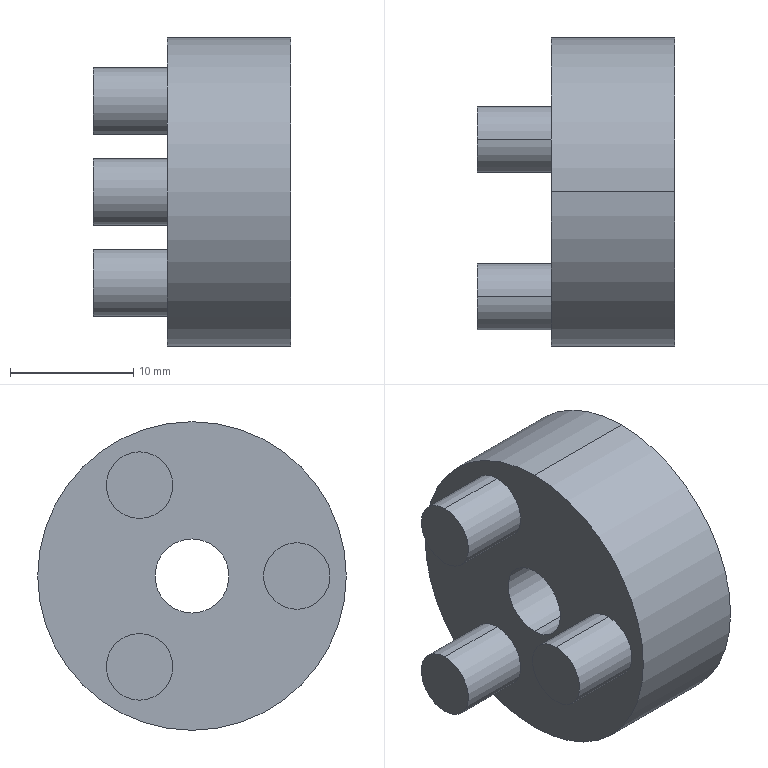Part | SolidWorks | features BaseBody 1 | 1 solid | 15 faces | box 16 x 25 x 25 mm | volume 5038 mm3 | cylinder 10 | plane 5 | commonest cylinder face diameters 5.4 x6 6 x2 25 x2
STEP:
#1=CARTESIAN_POINT('',(5.,0.,12.5));
#2=VERTEX_POINT('',#1);
#3=CARTESIAN_POINT('',(5.,0.,-12.5));
#4=VERTEX_POINT('',#3);
#5=CARTESIAN_POINT('',(5.,0.,0.));
#6=DIRECTION('',(-1.,0.,0.));
#7=DIRECTION('',(0.,0.,1.));
#8=AXIS2_PLACEMENT_3D('',#5,#6,#7);
#9=CIRCLE('',#8,12.5);
#10=EDGE_CURVE('',#2,#4,#9,.T.);
#11=ORIENTED_EDGE('',*,*,#10,.T.);
#12=CARTESIAN_POINT('',(-5.,0.,-12.5));
#13=VERTEX_POINT('',#12);
#14=CARTESIAN_POINT('',(5.,0.,-12.5));
#15=DIRECTION('',(-1.,0.,0.));
#16=VECTOR('',#15,1000.);
#17=LINE('',#14,#16);
#18=EDGE_CURVE('',#4,#13,#17,.T.);
#19=ORIENTED_EDGE('',*,*,#18,.T.);
#20=CARTESIAN_POINT('',(-5.,0.,12.5));
#21=VERTEX_POINT('',#20);
#22=CARTESIAN_POINT('',(-5.,0.,0.));
#23=DIRECTION('',(1.,0.,0.));
#24=DIRECTION('',(0.,0.,1.));
#25=AXIS2_PLACEMENT_3D('',#22,#23,#24);
#26=CIRCLE('',#25,12.5);
#27=EDGE_CURVE('',#13,#21,#26,.T.);
#28=ORIENTED_EDGE('',*,*,#27,.T.);
#29=CARTESIAN_POINT('',(5.,0.,12.5));
#30=DIRECTION('',(-1.,0.,0.));
#31=VECTOR('',#30,1000.);
#32=LINE('',#29,#31);
#33=EDGE_CURVE('',#2,#21,#32,.T.);
#34=ORIENTED_EDGE('',*,*,#33,.F.);
#35=EDGE_LOOP('',(#11,#19,#28,#34));
#36=FACE_OUTER_BOUND('',#35,.T.);
#37=CARTESIAN_POINT('',(5.,0.,0.));
#38=DIRECTION('',(-1.,0.,0.));
#39=DIRECTION('',(0.,0.,1.));
#40=AXIS2_PLACEMENT_3D('',#37,#38,#39);
#41=CYLINDRICAL_SURFACE('',#40,12.5);
#42=ADVANCED_FACE('',(#36),#41,.T.);
#43=CARTESIAN_POINT('',(-5.,0.,3.));
#44=VERTEX_POINT('',#43);
#45=CARTESIAN_POINT('',(-5.,0.,-3.));
#46=VERTEX_POINT('',#45);
#47=CARTESIAN_POINT('',(-5.,0.,0.));
#48=DIRECTION('',(1.,0.,0.));
#49=DIRECTION('',(0.,0.,-1.));
#50=AXIS2_PLACEMENT_3D('',#47,#48,#49);
#51=CIRCLE('',#50,3.);
#52=EDGE_CURVE('',#44,#46,#51,.T.);
#53=ORIENTED_EDGE('',*,*,#52,.F.);
#54=CARTESIAN_POINT('',(5.,0.,3.));
#55=VERTEX_POINT('',#54);
#56=CARTESIAN_POINT('',(-6.,0.,3.));
#57=DIRECTION('',(1.,0.,0.));
#58=VECTOR('',#57,1000.);
#59=LINE('',#56,#58);
#60=EDGE_CURVE('',#44,#55,#59,.T.);
#61=ORIENTED_EDGE('',*,*,#60,.T.);
#62=CARTESIAN_POINT('',(5.,0.,-3.));
#63=VERTEX_POINT('',#62);
#64=CARTESIAN_POINT('',(5.,0.,0.));
#65=DIRECTION('',(1.,0.,0.));
#66=DIRECTION('',(0.,0.,-1.));
#67=AXIS2_PLACEMENT_3D('',#64,#65,#66);
#68=CIRCLE('',#67,3.);
#69=EDGE_CURVE('',#55,#63,#68,.T.);
#70=ORIENTED_EDGE('',*,*,#69,.T.);
#71=CARTESIAN_POINT('',(-6.,0.,-3.));
#72=DIRECTION('',(1.,0.,0.));
#73=VECTOR('',#72,1000.);
#74=LINE('',#71,#73);
#75=EDGE_CURVE('',#46,#63,#74,.T.);
#76=ORIENTED_EDGE('',*,*,#75,.F.);
#77=EDGE_LOOP('',(#53,#61,#70,#76));
#78=FACE_OUTER_BOUND('',#77,.T.);
#79=CARTESIAN_POINT('',(-6.,0.,0.));
#80=DIRECTION('',(1.,0.,0.));
#81=DIRECTION('',(0.,0.,-1.));
#82=AXIS2_PLACEMENT_3D('',#79,#80,#81);
#83=CYLINDRICAL_SURFACE('',#82,3.);
#84=ADVANCED_FACE('',(#78),#83,.F.);
#85=CARTESIAN_POINT('',(-5.,4.25,-10.061));
#86=VERTEX_POINT('',#85);
#87=CARTESIAN_POINT('',(-5.,4.25,-4.661));
#88=VERTEX_POINT('',#87);
#89=CARTESIAN_POINT('',(-5.,4.25,-7.361));
#90=DIRECTION('',(1.,0.,0.));
#91=DIRECTION('',(0.,0.,1.));
#92=AXIS2_PLACEMENT_3D('',#89,#90,#91);
#93=CIRCLE('',#92,2.7);
#94=EDGE_CURVE('',#86,#88,#93,.T.);
#95=ORIENTED_EDGE('',*,*,#94,.F.);
#96=CARTESIAN_POINT('',(-11.,4.25,-10.061));
#97=VERTEX_POINT('',#96);
#98=CARTESIAN_POINT('',(-5.,4.25,-10.061));
#99=DIRECTION('',(-1.,0.,0.));
#100=VECTOR('',#99,1000.);
#101=LINE('',#98,#100);
#102=EDGE_CURVE('',#86,#97,#101,.T.);
#103=ORIENTED_EDGE('',*,*,#102,.T.);
#104=CARTESIAN_POINT('',(-11.,4.25,-4.661));
#105=VERTEX_POINT('',#104);
#106=CARTESIAN_POINT('',(-11.,4.25,-7.361));
#107=DIRECTION('',(1.,0.,0.));
#108=DIRECTION('',(0.,0.,1.));
#109=AXIS2_PLACEMENT_3D('',#106,#107,#108);
#110=CIRCLE('',#109,2.7);
#111=EDGE_CURVE('',#97,#105,#110,.T.);
#112=ORIENTED_EDGE('',*,*,#111,.T.);
#113=CARTESIAN_POINT('',(-5.,4.25,-4.661));
#114=DIRECTION('',(-1.,0.,0.));
#115=VECTOR('',#114,1000.);
#116=LINE('',#113,#115);
#117=EDGE_CURVE('',#88,#105,#116,.T.);
#118=ORIENTED_EDGE('',*,*,#117,.F.);
#119=EDGE_LOOP('',(#95,#103,#112,#118));
#120=FACE_OUTER_BOUND('',#119,.T.);
#121=CARTESIAN_POINT('',(-5.,4.25,-7.361));
#122=DIRECTION('',(-1.,0.,0.));
#123=DIRECTION('',(0.,0.,1.));
#124=AXIS2_PLACEMENT_3D('',#121,#122,#123);
#125=CYLINDRICAL_SURFACE('',#124,2.7);
#126=ADVANCED_FACE('',(#120),#125,.T.);
#127=CARTESIAN_POINT('',(-5.,4.25,4.661));
#128=VERTEX_POINT('',#127);
#129=CARTESIAN_POINT('',(-5.,4.25,10.061));
#130=VERTEX_POINT('',#129);
#131=CARTESIAN_POINT('',(-5.,4.25,7.361));
#132=DIRECTION('',(1.,0.,0.));
#133=DIRECTION('',(0.,0.,1.));
#134=AXIS2_PLACEMENT_3D('',#131,#132,#133);
#135=CIRCLE('',#134,2.7);
#136=EDGE_CURVE('',#128,#130,#135,.T.);
#137=ORIENTED_EDGE('',*,*,#136,.F.);
#138=CARTESIAN_POINT('',(-11.,4.25,4.661));
#139=VERTEX_POINT('',#138);
#140=CARTESIAN_POINT('',(-5.,4.25,4.661));
#141=DIRECTION('',(-1.,0.,0.));
#142=VECTOR('',#141,1000.);
#143=LINE('',#140,#142);
#144=EDGE_CURVE('',#128,#139,#143,.T.);
#145=ORIENTED_EDGE('',*,*,#144,.T.);
#146=CARTESIAN_POINT('',(-11.,4.25,10.061));
#147=VERTEX_POINT('',#146);
#148=CARTESIAN_POINT('',(-11.,4.25,7.361));
#149=DIRECTION('',(1.,0.,0.));
#150=DIRECTION('',(0.,0.,1.));
#151=AXIS2_PLACEMENT_3D('',#148,#149,#150);
#152=CIRCLE('',#151,2.7);
#153=EDGE_CURVE('',#139,#147,#152,.T.);
#154=ORIENTED_EDGE('',*,*,#153,.T.);
#155=CARTESIAN_POINT('',(-5.,4.25,10.061));
#156=DIRECTION('',(-1.,0.,0.));
#157=VECTOR('',#156,1000.);
#158=LINE('',#155,#157);
#159=EDGE_CURVE('',#130,#147,#158,.T.);
#160=ORIENTED_EDGE('',*,*,#159,.F.);
#161=EDGE_LOOP('',(#137,#145,#154,#160));
#162=FACE_OUTER_BOUND('',#161,.T.);
#163=CARTESIAN_POINT('',(-5.,4.25,7.361));
#164=DIRECTION('',(-1.,0.,0.));
#165=DIRECTION('',(0.,0.,1.));
#166=AXIS2_PLACEMENT_3D('',#163,#164,#165);
#167=CYLINDRICAL_SURFACE('',#166,2.7);
#168=ADVANCED_FACE('',(#162),#167,.T.);
#169=CARTESIAN_POINT('',(-5.,-8.5,-2.7));
#170=VERTEX_POINT('',#169);
#171=CARTESIAN_POINT('',(-5.,-8.5,2.7));
#172=VERTEX_POINT('',#171);
#173=CARTESIAN_POINT('',(-5.,-8.5,0.));
#174=DIRECTION('',(1.,0.,0.));
#175=DIRECTION('',(0.,0.,1.));
#176=AXIS2_PLACEMENT_3D('',#173,#174,#175);
#177=CIRCLE('',#176,2.7);
#178=EDGE_CURVE('',#170,#172,#177,.T.);
#179=ORIENTED_EDGE('',*,*,#178,.F.);
#180=CARTESIAN_POINT('',(-11.,-8.5,-2.7));
#181=VERTEX_POINT('',#180);
#182=CARTESIAN_POINT('',(-5.,-8.5,-2.7));
#183=DIRECTION('',(-1.,0.,0.));
#184=VECTOR('',#183,1000.);
#185=LINE('',#182,#184);
#186=EDGE_CURVE('',#170,#181,#185,.T.);
#187=ORIENTED_EDGE('',*,*,#186,.T.);
#188=CARTESIAN_POINT('',(-11.,-8.5,2.7));
#189=VERTEX_POINT('',#188);
#190=CARTESIAN_POINT('',(-11.,-8.5,0.));
#191=DIRECTION('',(1.,0.,0.));
#192=DIRECTION('',(0.,0.,1.));
#193=AXIS2_PLACEMENT_3D('',#190,#191,#192);
#194=CIRCLE('',#193,2.7);
#195=EDGE_CURVE('',#181,#189,#194,.T.);
#196=ORIENTED_EDGE('',*,*,#195,.T.);
#197=CARTESIAN_POINT('',(-5.,-8.5,2.7));
#198=DIRECTION('',(-1.,0.,0.));
#199=VECTOR('',#198,1000.);
#200=LINE('',#197,#199);
#201=EDGE_CURVE('',#172,#189,#200,.T.);
#202=ORIENTED_EDGE('',*,*,#201,.F.);
#203=EDGE_LOOP('',(#179,#187,#196,#202));
#204=FACE_OUTER_BOUND('',#203,.T.);
#205=CARTESIAN_POINT('',(-5.,-8.5,0.));
#206=DIRECTION('',(-1.,0.,0.));
#207=DIRECTION('',(0.,0.,1.));
#208=AXIS2_PLACEMENT_3D('',#205,#206,#207);
#209=CYLINDRICAL_SURFACE('',#208,2.7);
#210=ADVANCED_FACE('',(#204),#209,.T.);
#211=ORIENTED_EDGE('',*,*,#18,.F.);
#212=CARTESIAN_POINT('',(5.,0.,0.));
#213=DIRECTION('',(-1.,0.,0.));
#214=DIRECTION('',(0.,0.,1.));
#215=AXIS2_PLACEMENT_3D('',#212,#213,#214);
#216=CIRCLE('',#215,12.5);
#217=EDGE_CURVE('',#4,#2,#216,.T.);
#218=ORIENTED_EDGE('',*,*,#217,.T.);
#219=ORIENTED_EDGE('',*,*,#33,.T.);
#220=CARTESIAN_POINT('',(-5.,0.,0.));
#221=DIRECTION('',(1.,0.,0.));
#222=DIRECTION('',(0.,0.,1.));
#223=AXIS2_PLACEMENT_3D('',#220,#221,#222);
#224=CIRCLE('',#223,12.5);
#225=EDGE_CURVE('',#21,#13,#224,.T.);
#226=ORIENTED_EDGE('',*,*,#225,.T.);
#227=EDGE_LOOP('',(#211,#218,#219,#226));
#228=FACE_OUTER_BOUND('',#227,.T.);
#229=CARTESIAN_POINT('',(5.,0.,0.));
#230=DIRECTION('',(-1.,0.,0.));
#231=DIRECTION('',(0.,0.,1.));
#232=AXIS2_PLACEMENT_3D('',#229,#230,#231);
#233=CYLINDRICAL_SURFACE('',#232,12.5);
#234=ADVANCED_FACE('',(#228),#233,.T.);
#235=CARTESIAN_POINT('',(5.,0.,0.));
#236=DIRECTION('',(1.,0.,0.));
#237=DIRECTION('',(0.,0.,-1.));
#238=AXIS2_PLACEMENT_3D('',#235,#236,#237);
#239=CIRCLE('',#238,3.);
#240=EDGE_CURVE('',#63,#55,#239,.T.);
#241=ORIENTED_EDGE('',*,*,#240,.F.);
#242=ORIENTED_EDGE('',*,*,#69,.F.);
#243=EDGE_LOOP('',(#241,#242));
#244=FACE_BOUND('',#243,.T.);
#245=ORIENTED_EDGE('',*,*,#10,.F.);
#246=ORIENTED_EDGE('',*,*,#217,.F.);
#247=EDGE_LOOP('',(#245,#246));
#248=FACE_OUTER_BOUND('',#247,.T.);
#249=CARTESIAN_POINT('',(5.,0.,0.));
#250=DIRECTION('',(-1.,0.,0.));
#251=DIRECTION('',(0.,0.,1.));
#252=AXIS2_PLACEMENT_3D('',#249,#250,#251);
#253=PLANE('',#252);
#254=ADVANCED_FACE('',(#244,#248),#253,.F.);
#255=CARTESIAN_POINT('',(-5.,0.,0.));
#256=DIRECTION('',(1.,0.,0.));
#257=DIRECTION('',(0.,0.,-1.));
#258=AXIS2_PLACEMENT_3D('',#255,#256,#257);
#259=CIRCLE('',#258,3.);
#260=EDGE_CURVE('',#46,#44,#259,.T.);
#261=ORIENTED_EDGE('',*,*,#260,.T.);
#262=ORIENTED_EDGE('',*,*,#52,.T.);
#263=EDGE_LOOP('',(#261,#262));
#264=FACE_BOUND('',#263,.T.);
#265=CARTESIAN_POINT('',(-5.,4.25,-7.361));
#266=DIRECTION('',(1.,0.,0.));
#267=DIRECTION('',(0.,0.,1.));
#268=AXIS2_PLACEMENT_3D('',#265,#266,#267);
#269=CIRCLE('',#268,2.7);
#270=EDGE_CURVE('',#88,#86,#269,.T.);
#271=ORIENTED_EDGE('',*,*,#270,.T.);
#272=ORIENTED_EDGE('',*,*,#94,.T.);
#273=EDGE_LOOP('',(#271,#272));
#274=FACE_BOUND('',#273,.T.);
#275=CARTESIAN_POINT('',(-5.,4.25,7.361));
#276=DIRECTION('',(1.,0.,0.));
#277=DIRECTION('',(0.,0.,1.));
#278=AXIS2_PLACEMENT_3D('',#275,#276,#277);
#279=CIRCLE('',#278,2.7);
#280=EDGE_CURVE('',#130,#128,#279,.T.);
#281=ORIENTED_EDGE('',*,*,#280,.T.);
#282=ORIENTED_EDGE('',*,*,#136,.T.);
#283=EDGE_LOOP('',(#281,#282));
#284=FACE_BOUND('',#283,.T.);
#285=CARTESIAN_POINT('',(-5.,-8.5,0.));
#286=DIRECTION('',(1.,0.,0.));
#287=DIRECTION('',(0.,0.,1.));
#288=AXIS2_PLACEMENT_3D('',#285,#286,#287);
#289=CIRCLE('',#288,2.7);
#290=EDGE_CURVE('',#172,#170,#289,.T.);
#291=ORIENTED_EDGE('',*,*,#290,.T.);
#292=ORIENTED_EDGE('',*,*,#178,.T.);
#293=EDGE_LOOP('',(#291,#292));
#294=FACE_BOUND('',#293,.T.);
#295=ORIENTED_EDGE('',*,*,#225,.F.);
#296=ORIENTED_EDGE('',*,*,#27,.F.);
#297=EDGE_LOOP('',(#295,#296));
#298=FACE_OUTER_BOUND('',#297,.T.);
#299=CARTESIAN_POINT('',(-5.,0.,0.));
#300=DIRECTION('',(-1.,0.,0.));
#301=DIRECTION('',(0.,0.,1.));
#302=AXIS2_PLACEMENT_3D('',#299,#300,#301);
#303=PLANE('',#302);
#304=ADVANCED_FACE('',(#264,#274,#284,#294,#298),#303,.T.);
#305=ORIENTED_EDGE('',*,*,#60,.F.);
#306=ORIENTED_EDGE('',*,*,#260,.F.);
#307=ORIENTED_EDGE('',*,*,#75,.T.);
#308=ORIENTED_EDGE('',*,*,#240,.T.);
#309=EDGE_LOOP('',(#305,#306,#307,#308));
#310=FACE_OUTER_BOUND('',#309,.T.);
#311=CARTESIAN_POINT('',(-6.,0.,0.));
#312=DIRECTION('',(1.,0.,0.));
#313=DIRECTION('',(0.,0.,-1.));
#314=AXIS2_PLACEMENT_3D('',#311,#312,#313);
#315=CYLINDRICAL_SURFACE('',#314,3.);
#316=ADVANCED_FACE('',(#310),#315,.F.);
#317=ORIENTED_EDGE('',*,*,#102,.F.);
#318=ORIENTED_EDGE('',*,*,#270,.F.);
#319=ORIENTED_EDGE('',*,*,#117,.T.);
#320=CARTESIAN_POINT('',(-11.,4.25,-7.361));
#321=DIRECTION('',(1.,0.,0.));
#322=DIRECTION('',(0.,0.,1.));
#323=AXIS2_PLACEMENT_3D('',#320,#321,#322);
#324=CIRCLE('',#323,2.7);
#325=EDGE_CURVE('',#105,#97,#324,.T.);
#326=ORIENTED_EDGE('',*,*,#325,.T.);
#327=EDGE_LOOP('',(#317,#318,#319,#326));
#328=FACE_OUTER_BOUND('',#327,.T.);
#329=CARTESIAN_POINT('',(-5.,4.25,-7.361));
#330=DIRECTION('',(-1.,0.,0.));
#331=DIRECTION('',(0.,0.,1.));
#332=AXIS2_PLACEMENT_3D('',#329,#330,#331);
#333=CYLINDRICAL_SURFACE('',#332,2.7);
#334=ADVANCED_FACE('',(#328),#333,.T.);
#335=ORIENTED_EDGE('',*,*,#144,.F.);
#336=ORIENTED_EDGE('',*,*,#280,.F.);
#337=ORIENTED_EDGE('',*,*,#159,.T.);
#338=CARTESIAN_POINT('',(-11.,4.25,7.361));
#339=DIRECTION('',(1.,0.,0.));
#340=DIRECTION('',(0.,0.,1.));
#341=AXIS2_PLACEMENT_3D('',#338,#339,#340);
#342=CIRCLE('',#341,2.7);
#343=EDGE_CURVE('',#147,#139,#342,.T.);
#344=ORIENTED_EDGE('',*,*,#343,.T.);
#345=EDGE_LOOP('',(#335,#336,#337,#344));
#346=FACE_OUTER_BOUND('',#345,.T.);
#347=CARTESIAN_POINT('',(-5.,4.25,7.361));
#348=DIRECTION('',(-1.,0.,0.));
#349=DIRECTION('',(0.,0.,1.));
#350=AXIS2_PLACEMENT_3D('',#347,#348,#349);
#351=CYLINDRICAL_SURFACE('',#350,2.7);
#352=ADVANCED_FACE('',(#346),#351,.T.);
#353=ORIENTED_EDGE('',*,*,#186,.F.);
#354=ORIENTED_EDGE('',*,*,#290,.F.);
#355=ORIENTED_EDGE('',*,*,#201,.T.);
#356=CARTESIAN_POINT('',(-11.,-8.5,0.));
#357=DIRECTION('',(1.,0.,0.));
#358=DIRECTION('',(0.,0.,1.));
#359=AXIS2_PLACEMENT_3D('',#356,#357,#358);
#360=CIRCLE('',#359,2.7);
#361=EDGE_CURVE('',#189,#181,#360,.T.);
#362=ORIENTED_EDGE('',*,*,#361,.T.);
#363=EDGE_LOOP('',(#353,#354,#355,#362));
#364=FACE_OUTER_BOUND('',#363,.T.);
#365=CARTESIAN_POINT('',(-5.,-8.5,0.));
#366=DIRECTION('',(-1.,0.,0.));
#367=DIRECTION('',(0.,0.,1.));
#368=AXIS2_PLACEMENT_3D('',#365,#366,#367);
#369=CYLINDRICAL_SURFACE('',#368,2.7);
#370=ADVANCED_FACE('',(#364),#369,.T.);
#371=ORIENTED_EDGE('',*,*,#325,.F.);
#372=ORIENTED_EDGE('',*,*,#111,.F.);
#373=EDGE_LOOP('',(#371,#372));
#374=FACE_OUTER_BOUND('',#373,.T.);
#375=CARTESIAN_POINT('',(-11.,4.25,-7.361));
#376=DIRECTION('',(-1.,0.,0.));
#377=DIRECTION('',(0.,0.,1.));
#378=AXIS2_PLACEMENT_3D('',#375,#376,#377);
#379=PLANE('',#378);
#380=ADVANCED_FACE('',(#374),#379,.T.);
#381=ORIENTED_EDGE('',*,*,#343,.F.);
#382=ORIENTED_EDGE('',*,*,#153,.F.);
#383=EDGE_LOOP('',(#381,#382));
#384=FACE_OUTER_BOUND('',#383,.T.);
#385=CARTESIAN_POINT('',(-11.,4.25,7.361));
#386=DIRECTION('',(-1.,0.,0.));
#387=DIRECTION('',(0.,0.,1.));
#388=AXIS2_PLACEMENT_3D('',#385,#386,#387);
#389=PLANE('',#388);
#390=ADVANCED_FACE('',(#384),#389,.T.);
#391=ORIENTED_EDGE('',*,*,#361,.F.);
#392=ORIENTED_EDGE('',*,*,#195,.F.);
#393=EDGE_LOOP('',(#391,#392));
#394=FACE_OUTER_BOUND('',#393,.T.);
#395=CARTESIAN_POINT('',(-11.,-8.5,0.));
#396=DIRECTION('',(-1.,0.,0.));
#397=DIRECTION('',(0.,0.,1.));
#398=AXIS2_PLACEMENT_3D('',#395,#396,#397);
#399=PLANE('',#398);
#400=ADVANCED_FACE('',(#394),#399,.T.);
#401=CLOSED_SHELL('',(#42,#84,#126,#168,#210,#234,#254,#304,#316,#334,#352,#370,#380,#390,#400));
#402=MANIFOLD_SOLID_BREP('',#401);
#403=CARTESIAN_POINT('',(0.,0.,0.));
#404=DIRECTION('',(0.,0.,1.));
#405=DIRECTION('',(1.,0.,0.));
#406=AXIS2_PLACEMENT_3D('',#403,#404,#405);
#407=(LENGTH_UNIT()NAMED_UNIT(*)SI_UNIT(.MILLI.,.METRE.));
#408=UNCERTAINTY_MEASURE_WITH_UNIT(LENGTH_MEASURE(0.00001),#407,'','');
#409=(NAMED_UNIT(*)PLANE_ANGLE_UNIT()SI_UNIT($,.RADIAN.));
#410=(NAMED_UNIT(*)SI_UNIT($,.STERADIAN.)SOLID_ANGLE_UNIT());
#411=(GEOMETRIC_REPRESENTATION_CONTEXT(3)GLOBAL_UNCERTAINTY_ASSIGNED_CONTEXT((#408))GLOBAL_UNIT_ASSIGNED_CONTEXT((#407,#409,#410))REPRESENTATION_CONTEXT('',''));
#412=ADVANCED_BREP_SHAPE_REPRESENTATION('',(#402,#406),#411);